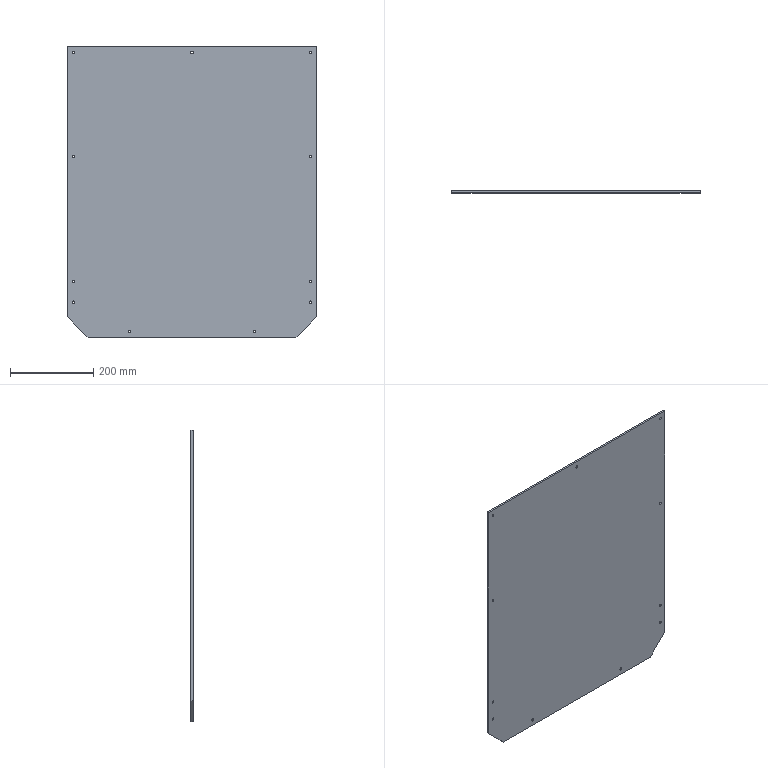Part | SolidWorks | features Extrusion 1, ICE 1 | 1 solid | 30 faces | box 600 x 5 x 700 mm | volume 2085945 mm3 | cylinder 22 | plane 8 | commonest cylinder face diameters 6 x22
STEP:
#1=CARTESIAN_POINT('',(300.,0.,-12.));
#2=VERTEX_POINT('',#1);
#3=CARTESIAN_POINT('',(300.,0.,-18.));
#4=VERTEX_POINT('',#3);
#5=CARTESIAN_POINT('',(300.,0.,-15.));
#6=DIRECTION('',(0.,-1.,0.));
#7=DIRECTION('',(0.,0.,-1.));
#8=AXIS2_PLACEMENT_3D('',#5,#6,#7);
#9=CIRCLE('',#8,3.);
#10=EDGE_CURVE('',#2,#4,#9,.T.);
#11=ORIENTED_EDGE('',*,*,#10,.T.);
#12=CARTESIAN_POINT('',(300.,5.,-18.));
#13=VERTEX_POINT('',#12);
#14=CARTESIAN_POINT('',(300.,-5.,-18.));
#15=DIRECTION('',(0.,1.,0.));
#16=VECTOR('',#15,1000.);
#17=LINE('',#14,#16);
#18=EDGE_CURVE('',#4,#13,#17,.T.);
#19=ORIENTED_EDGE('',*,*,#18,.T.);
#20=CARTESIAN_POINT('',(300.,5.,-12.));
#21=VERTEX_POINT('',#20);
#22=CARTESIAN_POINT('',(300.,5.,-15.));
#23=DIRECTION('',(0.,1.,0.));
#24=DIRECTION('',(0.,0.,1.));
#25=AXIS2_PLACEMENT_3D('',#22,#23,#24);
#26=CIRCLE('',#25,3.);
#27=EDGE_CURVE('',#13,#21,#26,.T.);
#28=ORIENTED_EDGE('',*,*,#27,.T.);
#29=CARTESIAN_POINT('',(300.,-5.,-12.));
#30=DIRECTION('',(0.,1.,0.));
#31=VECTOR('',#30,1000.);
#32=LINE('',#29,#31);
#33=EDGE_CURVE('',#2,#21,#32,.T.);
#34=ORIENTED_EDGE('',*,*,#33,.F.);
#35=EDGE_LOOP('',(#11,#19,#28,#34));
#36=FACE_OUTER_BOUND('',#35,.T.);
#37=CARTESIAN_POINT('',(300.,-5.,-15.));
#38=DIRECTION('',(0.,1.,0.));
#39=DIRECTION('',(0.,0.,1.));
#40=AXIS2_PLACEMENT_3D('',#37,#38,#39);
#41=CYLINDRICAL_SURFACE('',#40,3.);
#42=ADVANCED_FACE('',(#36),#41,.F.);
#43=CARTESIAN_POINT('',(450.,0.,-682.));
#44=VERTEX_POINT('',#43);
#45=CARTESIAN_POINT('',(450.,0.,-688.));
#46=VERTEX_POINT('',#45);
#47=CARTESIAN_POINT('',(450.,0.,-685.));
#48=DIRECTION('',(0.,-1.,0.));
#49=DIRECTION('',(0.,0.,-1.));
#50=AXIS2_PLACEMENT_3D('',#47,#48,#49);
#51=CIRCLE('',#50,3.);
#52=EDGE_CURVE('',#44,#46,#51,.T.);
#53=ORIENTED_EDGE('',*,*,#52,.T.);
#54=CARTESIAN_POINT('',(450.,5.,-688.));
#55=VERTEX_POINT('',#54);
#56=CARTESIAN_POINT('',(450.,-5.,-688.));
#57=DIRECTION('',(0.,1.,0.));
#58=VECTOR('',#57,1000.);
#59=LINE('',#56,#58);
#60=EDGE_CURVE('',#46,#55,#59,.T.);
#61=ORIENTED_EDGE('',*,*,#60,.T.);
#62=CARTESIAN_POINT('',(450.,5.,-682.));
#63=VERTEX_POINT('',#62);
#64=CARTESIAN_POINT('',(450.,5.,-685.));
#65=DIRECTION('',(0.,1.,0.));
#66=DIRECTION('',(0.,0.,-1.));
#67=AXIS2_PLACEMENT_3D('',#64,#65,#66);
#68=CIRCLE('',#67,3.);
#69=EDGE_CURVE('',#55,#63,#68,.T.);
#70=ORIENTED_EDGE('',*,*,#69,.T.);
#71=CARTESIAN_POINT('',(450.,-5.,-682.));
#72=DIRECTION('',(0.,1.,0.));
#73=VECTOR('',#72,1000.);
#74=LINE('',#71,#73);
#75=EDGE_CURVE('',#44,#63,#74,.T.);
#76=ORIENTED_EDGE('',*,*,#75,.F.);
#77=EDGE_LOOP('',(#53,#61,#70,#76));
#78=FACE_OUTER_BOUND('',#77,.T.);
#79=CARTESIAN_POINT('',(450.,-5.,-685.));
#80=DIRECTION('',(0.,1.,0.));
#81=DIRECTION('',(0.,0.,1.));
#82=AXIS2_PLACEMENT_3D('',#79,#80,#81);
#83=CYLINDRICAL_SURFACE('',#82,3.);
#84=ADVANCED_FACE('',(#78),#83,.F.);
#85=CARTESIAN_POINT('',(585.,0.,-612.));
#86=VERTEX_POINT('',#85);
#87=CARTESIAN_POINT('',(585.,0.,-618.));
#88=VERTEX_POINT('',#87);
#89=CARTESIAN_POINT('',(585.,0.,-615.));
#90=DIRECTION('',(0.,-1.,0.));
#91=DIRECTION('',(0.,0.,-1.));
#92=AXIS2_PLACEMENT_3D('',#89,#90,#91);
#93=CIRCLE('',#92,3.);
#94=EDGE_CURVE('',#86,#88,#93,.T.);
#95=ORIENTED_EDGE('',*,*,#94,.T.);
#96=CARTESIAN_POINT('',(585.,5.,-618.));
#97=VERTEX_POINT('',#96);
#98=CARTESIAN_POINT('',(585.,-5.,-618.));
#99=DIRECTION('',(0.,1.,0.));
#100=VECTOR('',#99,1000.);
#101=LINE('',#98,#100);
#102=EDGE_CURVE('',#88,#97,#101,.T.);
#103=ORIENTED_EDGE('',*,*,#102,.T.);
#104=CARTESIAN_POINT('',(585.,5.,-612.));
#105=VERTEX_POINT('',#104);
#106=CARTESIAN_POINT('',(585.,5.,-615.));
#107=DIRECTION('',(0.,1.,0.));
#108=DIRECTION('',(0.,0.,-1.));
#109=AXIS2_PLACEMENT_3D('',#106,#107,#108);
#110=CIRCLE('',#109,3.);
#111=EDGE_CURVE('',#97,#105,#110,.T.);
#112=ORIENTED_EDGE('',*,*,#111,.T.);
#113=CARTESIAN_POINT('',(585.,-5.,-612.));
#114=DIRECTION('',(0.,1.,0.));
#115=VECTOR('',#114,1000.);
#116=LINE('',#113,#115);
#117=EDGE_CURVE('',#86,#105,#116,.T.);
#118=ORIENTED_EDGE('',*,*,#117,.F.);
#119=EDGE_LOOP('',(#95,#103,#112,#118));
#120=FACE_OUTER_BOUND('',#119,.T.);
#121=CARTESIAN_POINT('',(585.,-5.,-615.));
#122=DIRECTION('',(0.,1.,0.));
#123=DIRECTION('',(0.,0.,1.));
#124=AXIS2_PLACEMENT_3D('',#121,#122,#123);
#125=CYLINDRICAL_SURFACE('',#124,3.);
#126=ADVANCED_FACE('',(#120),#125,.F.);
#127=CARTESIAN_POINT('',(585.,0.,-562.));
#128=VERTEX_POINT('',#127);
#129=CARTESIAN_POINT('',(585.,0.,-568.));
#130=VERTEX_POINT('',#129);
#131=CARTESIAN_POINT('',(585.,0.,-565.));
#132=DIRECTION('',(0.,-1.,0.));
#133=DIRECTION('',(0.,0.,-1.));
#134=AXIS2_PLACEMENT_3D('',#131,#132,#133);
#135=CIRCLE('',#134,3.);
#136=EDGE_CURVE('',#128,#130,#135,.T.);
#137=ORIENTED_EDGE('',*,*,#136,.T.);
#138=CARTESIAN_POINT('',(585.,5.,-568.));
#139=VERTEX_POINT('',#138);
#140=CARTESIAN_POINT('',(585.,-5.,-568.));
#141=DIRECTION('',(0.,1.,0.));
#142=VECTOR('',#141,1000.);
#143=LINE('',#140,#142);
#144=EDGE_CURVE('',#130,#139,#143,.T.);
#145=ORIENTED_EDGE('',*,*,#144,.T.);
#146=CARTESIAN_POINT('',(585.,5.,-562.));
#147=VERTEX_POINT('',#146);
#148=CARTESIAN_POINT('',(585.,5.,-565.));
#149=DIRECTION('',(0.,1.,0.));
#150=DIRECTION('',(0.,0.,-1.));
#151=AXIS2_PLACEMENT_3D('',#148,#149,#150);
#152=CIRCLE('',#151,3.);
#153=EDGE_CURVE('',#139,#147,#152,.T.);
#154=ORIENTED_EDGE('',*,*,#153,.T.);
#155=CARTESIAN_POINT('',(585.,-5.,-562.));
#156=DIRECTION('',(0.,1.,0.));
#157=VECTOR('',#156,1000.);
#158=LINE('',#155,#157);
#159=EDGE_CURVE('',#128,#147,#158,.T.);
#160=ORIENTED_EDGE('',*,*,#159,.F.);
#161=EDGE_LOOP('',(#137,#145,#154,#160));
#162=FACE_OUTER_BOUND('',#161,.T.);
#163=CARTESIAN_POINT('',(585.,-5.,-565.));
#164=DIRECTION('',(0.,1.,0.));
#165=DIRECTION('',(0.,0.,1.));
#166=AXIS2_PLACEMENT_3D('',#163,#164,#165);
#167=CYLINDRICAL_SURFACE('',#166,3.);
#168=ADVANCED_FACE('',(#162),#167,.F.);
#169=CARTESIAN_POINT('',(585.,0.,-262.));
#170=VERTEX_POINT('',#169);
#171=CARTESIAN_POINT('',(585.,0.,-268.));
#172=VERTEX_POINT('',#171);
#173=CARTESIAN_POINT('',(585.,0.,-265.));
#174=DIRECTION('',(0.,-1.,0.));
#175=DIRECTION('',(0.,0.,-1.));
#176=AXIS2_PLACEMENT_3D('',#173,#174,#175);
#177=CIRCLE('',#176,3.);
#178=EDGE_CURVE('',#170,#172,#177,.T.);
#179=ORIENTED_EDGE('',*,*,#178,.T.);
#180=CARTESIAN_POINT('',(585.,5.,-268.));
#181=VERTEX_POINT('',#180);
#182=CARTESIAN_POINT('',(585.,-5.,-268.));
#183=DIRECTION('',(0.,1.,0.));
#184=VECTOR('',#183,1000.);
#185=LINE('',#182,#184);
#186=EDGE_CURVE('',#172,#181,#185,.T.);
#187=ORIENTED_EDGE('',*,*,#186,.T.);
#188=CARTESIAN_POINT('',(585.,5.,-262.));
#189=VERTEX_POINT('',#188);
#190=CARTESIAN_POINT('',(585.,5.,-265.));
#191=DIRECTION('',(0.,1.,0.));
#192=DIRECTION('',(0.,0.,-1.));
#193=AXIS2_PLACEMENT_3D('',#190,#191,#192);
#194=CIRCLE('',#193,3.);
#195=EDGE_CURVE('',#181,#189,#194,.T.);
#196=ORIENTED_EDGE('',*,*,#195,.T.);
#197=CARTESIAN_POINT('',(585.,-5.,-262.));
#198=DIRECTION('',(0.,1.,0.));
#199=VECTOR('',#198,1000.);
#200=LINE('',#197,#199);
#201=EDGE_CURVE('',#170,#189,#200,.T.);
#202=ORIENTED_EDGE('',*,*,#201,.F.);
#203=EDGE_LOOP('',(#179,#187,#196,#202));
#204=FACE_OUTER_BOUND('',#203,.T.);
#205=CARTESIAN_POINT('',(585.,-5.,-265.));
#206=DIRECTION('',(0.,1.,0.));
#207=DIRECTION('',(0.,0.,1.));
#208=AXIS2_PLACEMENT_3D('',#205,#206,#207);
#209=CYLINDRICAL_SURFACE('',#208,3.);
#210=ADVANCED_FACE('',(#204),#209,.F.);
#211=CARTESIAN_POINT('',(585.,0.,-12.));
#212=VERTEX_POINT('',#211);
#213=CARTESIAN_POINT('',(585.,0.,-18.));
#214=VERTEX_POINT('',#213);
#215=CARTESIAN_POINT('',(585.,0.,-15.));
#216=DIRECTION('',(0.,-1.,0.));
#217=DIRECTION('',(0.,0.,-1.));
#218=AXIS2_PLACEMENT_3D('',#215,#216,#217);
#219=CIRCLE('',#218,3.);
#220=EDGE_CURVE('',#212,#214,#219,.T.);
#221=ORIENTED_EDGE('',*,*,#220,.T.);
#222=CARTESIAN_POINT('',(585.,5.,-18.));
#223=VERTEX_POINT('',#222);
#224=CARTESIAN_POINT('',(585.,-5.,-18.));
#225=DIRECTION('',(0.,1.,0.));
#226=VECTOR('',#225,1000.);
#227=LINE('',#224,#226);
#228=EDGE_CURVE('',#214,#223,#227,.T.);
#229=ORIENTED_EDGE('',*,*,#228,.T.);
#230=CARTESIAN_POINT('',(585.,5.,-12.));
#231=VERTEX_POINT('',#230);
#232=CARTESIAN_POINT('',(585.,5.,-15.));
#233=DIRECTION('',(0.,1.,0.));
#234=DIRECTION('',(0.,0.,-1.));
#235=AXIS2_PLACEMENT_3D('',#232,#233,#234);
#236=CIRCLE('',#235,3.);
#237=EDGE_CURVE('',#223,#231,#236,.T.);
#238=ORIENTED_EDGE('',*,*,#237,.T.);
#239=CARTESIAN_POINT('',(585.,-5.,-12.));
#240=DIRECTION('',(0.,1.,0.));
#241=VECTOR('',#240,1000.);
#242=LINE('',#239,#241);
#243=EDGE_CURVE('',#212,#231,#242,.T.);
#244=ORIENTED_EDGE('',*,*,#243,.F.);
#245=EDGE_LOOP('',(#221,#229,#238,#244));
#246=FACE_OUTER_BOUND('',#245,.T.);
#247=CARTESIAN_POINT('',(585.,-5.,-15.));
#248=DIRECTION('',(0.,1.,0.));
#249=DIRECTION('',(0.,0.,1.));
#250=AXIS2_PLACEMENT_3D('',#247,#248,#249);
#251=CYLINDRICAL_SURFACE('',#250,3.);
#252=ADVANCED_FACE('',(#246),#251,.F.);
#253=CARTESIAN_POINT('',(150.,0.,-682.));
#254=VERTEX_POINT('',#253);
#255=CARTESIAN_POINT('',(150.,0.,-688.));
#256=VERTEX_POINT('',#255);
#257=CARTESIAN_POINT('',(150.,0.,-685.));
#258=DIRECTION('',(0.,-1.,0.));
#259=DIRECTION('',(0.,0.,-1.));
#260=AXIS2_PLACEMENT_3D('',#257,#258,#259);
#261=CIRCLE('',#260,3.);
#262=EDGE_CURVE('',#254,#256,#261,.T.);
#263=ORIENTED_EDGE('',*,*,#262,.T.);
#264=CARTESIAN_POINT('',(150.,5.,-688.));
#265=VERTEX_POINT('',#264);
#266=CARTESIAN_POINT('',(150.,-5.,-688.));
#267=DIRECTION('',(0.,1.,0.));
#268=VECTOR('',#267,1000.);
#269=LINE('',#266,#268);
#270=EDGE_CURVE('',#256,#265,#269,.T.);
#271=ORIENTED_EDGE('',*,*,#270,.T.);
#272=CARTESIAN_POINT('',(150.,5.,-682.));
#273=VERTEX_POINT('',#272);
#274=CARTESIAN_POINT('',(150.,5.,-685.));
#275=DIRECTION('',(0.,1.,0.));
#276=DIRECTION('',(0.,0.,1.));
#277=AXIS2_PLACEMENT_3D('',#274,#275,#276);
#278=CIRCLE('',#277,3.);
#279=EDGE_CURVE('',#265,#273,#278,.T.);
#280=ORIENTED_EDGE('',*,*,#279,.T.);
#281=CARTESIAN_POINT('',(150.,-5.,-682.));
#282=DIRECTION('',(0.,1.,0.));
#283=VECTOR('',#282,1000.);
#284=LINE('',#281,#283);
#285=EDGE_CURVE('',#254,#273,#284,.T.);
#286=ORIENTED_EDGE('',*,*,#285,.F.);
#287=EDGE_LOOP('',(#263,#271,#280,#286));
#288=FACE_OUTER_BOUND('',#287,.T.);
#289=CARTESIAN_POINT('',(150.,-5.,-685.));
#290=DIRECTION('',(0.,1.,0.));
#291=DIRECTION('',(0.,0.,1.));
#292=AXIS2_PLACEMENT_3D('',#289,#290,#291);
#293=CYLINDRICAL_SURFACE('',#292,3.);
#294=ADVANCED_FACE('',(#288),#293,.F.);
#295=CARTESIAN_POINT('',(15.,0.,-612.));
#296=VERTEX_POINT('',#295);
#297=CARTESIAN_POINT('',(15.,0.,-618.));
#298=VERTEX_POINT('',#297);
#299=CARTESIAN_POINT('',(15.,0.,-615.));
#300=DIRECTION('',(0.,-1.,0.));
#301=DIRECTION('',(0.,0.,-1.));
#302=AXIS2_PLACEMENT_3D('',#299,#300,#301);
#303=CIRCLE('',#302,3.);
#304=EDGE_CURVE('',#296,#298,#303,.T.);
#305=ORIENTED_EDGE('',*,*,#304,.T.);
#306=CARTESIAN_POINT('',(15.,5.,-618.));
#307=VERTEX_POINT('',#306);
#308=CARTESIAN_POINT('',(15.,-5.,-618.));
#309=DIRECTION('',(0.,1.,0.));
#310=VECTOR('',#309,1000.);
#311=LINE('',#308,#310);
#312=EDGE_CURVE('',#298,#307,#311,.T.);
#313=ORIENTED_EDGE('',*,*,#312,.T.);
#314=CARTESIAN_POINT('',(15.,5.,-612.));
#315=VERTEX_POINT('',#314);
#316=CARTESIAN_POINT('',(15.,5.,-615.));
#317=DIRECTION('',(0.,1.,0.));
#318=DIRECTION('',(0.,0.,1.));
#319=AXIS2_PLACEMENT_3D('',#316,#317,#318);
#320=CIRCLE('',#319,3.);
#321=EDGE_CURVE('',#307,#315,#320,.T.);
#322=ORIENTED_EDGE('',*,*,#321,.T.);
#323=CARTESIAN_POINT('',(15.,-5.,-612.));
#324=DIRECTION('',(0.,1.,0.));
#325=VECTOR('',#324,1000.);
#326=LINE('',#323,#325);
#327=EDGE_CURVE('',#296,#315,#326,.T.);
#328=ORIENTED_EDGE('',*,*,#327,.F.);
#329=EDGE_LOOP('',(#305,#313,#322,#328));
#330=FACE_OUTER_BOUND('',#329,.T.);
#331=CARTESIAN_POINT('',(15.,-5.,-615.));
#332=DIRECTION('',(0.,1.,0.));
#333=DIRECTION('',(0.,0.,1.));
#334=AXIS2_PLACEMENT_3D('',#331,#332,#333);
#335=CYLINDRICAL_SURFACE('',#334,3.);
#336=ADVANCED_FACE('',(#330),#335,.F.);
#337=CARTESIAN_POINT('',(15.,0.,-562.));
#338=VERTEX_POINT('',#337);
#339=CARTESIAN_POINT('',(15.,0.,-568.));
#340=VERTEX_POINT('',#339);
#341=CARTESIAN_POINT('',(15.,0.,-565.));
#342=DIRECTION('',(0.,-1.,0.));
#343=DIRECTION('',(0.,0.,-1.));
#344=AXIS2_PLACEMENT_3D('',#341,#342,#343);
#345=CIRCLE('',#344,3.);
#346=EDGE_CURVE('',#338,#340,#345,.T.);
#347=ORIENTED_EDGE('',*,*,#346,.T.);
#348=CARTESIAN_POINT('',(15.,5.,-568.));
#349=VERTEX_POINT('',#348);
#350=CARTESIAN_POINT('',(15.,-5.,-568.));
#351=DIRECTION('',(0.,1.,0.));
#352=VECTOR('',#351,1000.);
#353=LINE('',#350,#352);
#354=EDGE_CURVE('',#340,#349,#353,.T.);
#355=ORIENTED_EDGE('',*,*,#354,.T.);
#356=CARTESIAN_POINT('',(15.,5.,-562.));
#357=VERTEX_POINT('',#356);
#358=CARTESIAN_POINT('',(15.,5.,-565.));
#359=DIRECTION('',(0.,1.,0.));
#360=DIRECTION('',(0.,0.,1.));
#361=AXIS2_PLACEMENT_3D('',#358,#359,#360);
#362=CIRCLE('',#361,3.);
#363=EDGE_CURVE('',#349,#357,#362,.T.);
#364=ORIENTED_EDGE('',*,*,#363,.T.);
#365=CARTESIAN_POINT('',(15.,-5.,-562.));
#366=DIRECTION('',(0.,1.,0.));
#367=VECTOR('',#366,1000.);
#368=LINE('',#365,#367);
#369=EDGE_CURVE('',#338,#357,#368,.T.);
#370=ORIENTED_EDGE('',*,*,#369,.F.);
#371=EDGE_LOOP('',(#347,#355,#364,#370));
#372=FACE_OUTER_BOUND('',#371,.T.);
#373=CARTESIAN_POINT('',(15.,-5.,-565.));
#374=DIRECTION('',(0.,1.,0.));
#375=DIRECTION('',(0.,0.,1.));
#376=AXIS2_PLACEMENT_3D('',#373,#374,#375);
#377=CYLINDRICAL_SURFACE('',#376,3.);
#378=ADVANCED_FACE('',(#372),#377,.F.);
#379=CARTESIAN_POINT('',(15.,0.,-262.));
#380=VERTEX_POINT('',#379);
#381=CARTESIAN_POINT('',(15.,0.,-268.));
#382=VERTEX_POINT('',#381);
#383=CARTESIAN_POINT('',(15.,0.,-265.));
#384=DIRECTION('',(0.,-1.,0.));
#385=DIRECTION('',(0.,0.,-1.));
#386=AXIS2_PLACEMENT_3D('',#383,#384,#385);
#387=CIRCLE('',#386,3.);
#388=EDGE_CURVE('',#380,#382,#387,.T.);
#389=ORIENTED_EDGE('',*,*,#388,.T.);
#390=CARTESIAN_POINT('',(15.,5.,-268.));
#391=VERTEX_POINT('',#390);
#392=CARTESIAN_POINT('',(15.,-5.,-268.));
#393=DIRECTION('',(0.,1.,0.));
#394=VECTOR('',#393,1000.);
#395=LINE('',#392,#394);
#396=EDGE_CURVE('',#382,#391,#395,.T.);
#397=ORIENTED_EDGE('',*,*,#396,.T.);
#398=CARTESIAN_POINT('',(15.,5.,-262.));
#399=VERTEX_POINT('',#398);
#400=CARTESIAN_POINT('',(15.,5.,-265.));
#401=DIRECTION('',(0.,1.,0.));
#402=DIRECTION('',(0.,0.,1.));
#403=AXIS2_PLACEMENT_3D('',#400,#401,#402);
#404=CIRCLE('',#403,3.);
#405=EDGE_CURVE('',#391,#399,#404,.T.);
#406=ORIENTED_EDGE('',*,*,#405,.T.);
#407=CARTESIAN_POINT('',(15.,-5.,-262.));
#408=DIRECTION('',(0.,1.,0.));
#409=VECTOR('',#408,1000.);
#410=LINE('',#407,#409);
#411=EDGE_CURVE('',#380,#399,#410,.T.);
#412=ORIENTED_EDGE('',*,*,#411,.F.);
#413=EDGE_LOOP('',(#389,#397,#406,#412));
#414=FACE_OUTER_BOUND('',#413,.T.);
#415=CARTESIAN_POINT('',(15.,-5.,-265.));
#416=DIRECTION('',(0.,1.,0.));
#417=DIRECTION('',(0.,0.,1.));
#418=AXIS2_PLACEMENT_3D('',#415,#416,#417);
#419=CYLINDRICAL_SURFACE('',#418,3.);
#420=ADVANCED_FACE('',(#414),#419,.F.);
#421=CARTESIAN_POINT('',(15.,0.,-12.));
#422=VERTEX_POINT('',#421);
#423=CARTESIAN_POINT('',(15.,0.,-18.));
#424=VERTEX_POINT('',#423);
#425=CARTESIAN_POINT('',(15.,0.,-15.));
#426=DIRECTION('',(0.,-1.,0.));
#427=DIRECTION('',(0.,0.,-1.));
#428=AXIS2_PLACEMENT_3D('',#425,#426,#427);
#429=CIRCLE('',#428,3.);
#430=EDGE_CURVE('',#422,#424,#429,.T.);
#431=ORIENTED_EDGE('',*,*,#430,.T.);
#432=CARTESIAN_POINT('',(15.,5.,-18.));
#433=VERTEX_POINT('',#432);
#434=CARTESIAN_POINT('',(15.,-5.,-18.));
#435=DIRECTION('',(0.,1.,0.));
#436=VECTOR('',#435,1000.);
#437=LINE('',#434,#436);
#438=EDGE_CURVE('',#424,#433,#437,.T.);
#439=ORIENTED_EDGE('',*,*,#438,.T.);
#440=CARTESIAN_POINT('',(15.,5.,-12.));
#441=VERTEX_POINT('',#440);
#442=CARTESIAN_POINT('',(15.,5.,-15.));
#443=DIRECTION('',(0.,1.,0.));
#444=DIRECTION('',(0.,0.,1.));
#445=AXIS2_PLACEMENT_3D('',#442,#443,#444);
#446=CIRCLE('',#445,3.);
#447=EDGE_CURVE('',#433,#441,#446,.T.);
#448=ORIENTED_EDGE('',*,*,#447,.T.);
#449=CARTESIAN_POINT('',(15.,-5.,-12.));
#450=DIRECTION('',(0.,1.,0.));
#451=VECTOR('',#450,1000.);
#452=LINE('',#449,#451);
#453=EDGE_CURVE('',#422,#441,#452,.T.);
#454=ORIENTED_EDGE('',*,*,#453,.F.);
#455=EDGE_LOOP('',(#431,#439,#448,#454));
#456=FACE_OUTER_BOUND('',#455,.T.);
#457=CARTESIAN_POINT('',(15.,-5.,-15.));
#458=DIRECTION('',(0.,1.,0.));
#459=DIRECTION('',(0.,0.,1.));
#460=AXIS2_PLACEMENT_3D('',#457,#458,#459);
#461=CYLINDRICAL_SURFACE('',#460,3.);
#462=ADVANCED_FACE('',(#456),#461,.F.);
#463=CARTESIAN_POINT('',(0.,0.,-650.));
#464=VERTEX_POINT('',#463);
#465=CARTESIAN_POINT('',(0.,0.,0.));
#466=VERTEX_POINT('',#465);
#467=CARTESIAN_POINT('',(0.,0.,0.));
#468=DIRECTION('',(0.,0.,1.));
#469=VECTOR('',#468,1000.);
#470=LINE('',#467,#469);
#471=EDGE_CURVE('',#464,#466,#470,.T.);
#472=ORIENTED_EDGE('',*,*,#471,.T.);
#473=CARTESIAN_POINT('',(0.,5.,0.));
#474=VERTEX_POINT('',#473);
#475=CARTESIAN_POINT('',(0.,5.,0.));
#476=DIRECTION('',(0.,-1.,0.));
#477=VECTOR('',#476,1000.);
#478=LINE('',#475,#477);
#479=EDGE_CURVE('',#474,#466,#478,.T.);
#480=ORIENTED_EDGE('',*,*,#479,.F.);
#481=CARTESIAN_POINT('',(0.,5.,-650.));
#482=VERTEX_POINT('',#481);
#483=CARTESIAN_POINT('',(0.,5.,0.));
#484=DIRECTION('',(0.,0.,1.));
#485=VECTOR('',#484,1000.);
#486=LINE('',#483,#485);
#487=EDGE_CURVE('',#482,#474,#486,.T.);
#488=ORIENTED_EDGE('',*,*,#487,.F.);
#489=CARTESIAN_POINT('',(0.,5.,-650.));
#490=DIRECTION('',(0.,-1.,0.));
#491=VECTOR('',#490,1000.);
#492=LINE('',#489,#491);
#493=EDGE_CURVE('',#482,#464,#492,.T.);
#494=ORIENTED_EDGE('',*,*,#493,.T.);
#495=EDGE_LOOP('',(#472,#480,#488,#494));
#496=FACE_OUTER_BOUND('',#495,.T.);
#497=CARTESIAN_POINT('',(0.,5.,0.));
#498=DIRECTION('',(1.,0.,0.));
#499=DIRECTION('',(0.,0.,-1.));
#500=AXIS2_PLACEMENT_3D('',#497,#498,#499);
#501=PLANE('',#500);
#502=ADVANCED_FACE('',(#496),#501,.F.);
#503=CARTESIAN_POINT('',(600.,0.,0.));
#504=VERTEX_POINT('',#503);
#505=CARTESIAN_POINT('',(0.,0.,0.));
#506=DIRECTION('',(1.,0.,0.));
#507=VECTOR('',#506,1000.);
#508=LINE('',#505,#507);
#509=EDGE_CURVE('',#466,#504,#508,.T.);
#510=ORIENTED_EDGE('',*,*,#509,.T.);
#511=CARTESIAN_POINT('',(600.,5.,0.));
#512=VERTEX_POINT('',#511);
#513=CARTESIAN_POINT('',(600.,5.,0.));
#514=DIRECTION('',(0.,-1.,0.));
#515=VECTOR('',#514,1000.);
#516=LINE('',#513,#515);
#517=EDGE_CURVE('',#512,#504,#516,.T.);
#518=ORIENTED_EDGE('',*,*,#517,.F.);
#519=CARTESIAN_POINT('',(0.,5.,0.));
#520=DIRECTION('',(1.,0.,0.));
#521=VECTOR('',#520,1000.);
#522=LINE('',#519,#521);
#523=EDGE_CURVE('',#474,#512,#522,.T.);
#524=ORIENTED_EDGE('',*,*,#523,.F.);
#525=ORIENTED_EDGE('',*,*,#479,.T.);
#526=EDGE_LOOP('',(#510,#518,#524,#525));
#527=FACE_OUTER_BOUND('',#526,.T.);
#528=CARTESIAN_POINT('',(0.,5.,0.));
#529=DIRECTION('',(0.,0.,-1.));
#530=DIRECTION('',(-1.,0.,0.));
#531=AXIS2_PLACEMENT_3D('',#528,#529,#530);
#532=PLANE('',#531);
#533=ADVANCED_FACE('',(#527),#532,.F.);
#534=CARTESIAN_POINT('',(600.,0.,-650.));
#535=VERTEX_POINT('',#534);
#536=CARTESIAN_POINT('',(600.,0.,0.));
#537=DIRECTION('',(0.,0.,-1.));
#538=VECTOR('',#537,1000.);
#539=LINE('',#536,#538);
#540=EDGE_CURVE('',#504,#535,#539,.T.);
#541=ORIENTED_EDGE('',*,*,#540,.T.);
#542=CARTESIAN_POINT('',(600.,5.,-650.));
#543=VERTEX_POINT('',#542);
#544=CARTESIAN_POINT('',(600.,5.,-650.));
#545=DIRECTION('',(0.,-1.,0.));
#546=VECTOR('',#545,1000.);
#547=LINE('',#544,#546);
#548=EDGE_CURVE('',#543,#535,#547,.T.);
#549=ORIENTED_EDGE('',*,*,#548,.F.);
#550=CARTESIAN_POINT('',(600.,5.,0.));
#551=DIRECTION('',(0.,0.,-1.));
#552=VECTOR('',#551,1000.);
#553=LINE('',#550,#552);
#554=EDGE_CURVE('',#512,#543,#553,.T.);
#555=ORIENTED_EDGE('',*,*,#554,.F.);
#556=ORIENTED_EDGE('',*,*,#517,.T.);
#557=EDGE_LOOP('',(#541,#549,#555,#556));
#558=FACE_OUTER_BOUND('',#557,.T.);
#559=CARTESIAN_POINT('',(600.,5.,0.));
#560=DIRECTION('',(-1.,0.,0.));
#561=DIRECTION('',(0.,0.,1.));
#562=AXIS2_PLACEMENT_3D('',#559,#560,#561);
#563=PLANE('',#562);
#564=ADVANCED_FACE('',(#558),#563,.F.);
#565=CARTESIAN_POINT('',(550.,0.,-700.));
#566=VERTEX_POINT('',#565);
#567=CARTESIAN_POINT('',(550.,0.,-700.));
#568=DIRECTION('',(-0.7071,0.,-0.7071));
#569=VECTOR('',#568,1000.);
#570=LINE('',#567,#569);
#571=EDGE_CURVE('',#535,#566,#570,.T.);
#572=ORIENTED_EDGE('',*,*,#571,.T.);
#573=CARTESIAN_POINT('',(550.,5.,-700.));
#574=VERTEX_POINT('',#573);
#575=CARTESIAN_POINT('',(550.,5.,-700.));
#576=DIRECTION('',(0.,-1.,0.));
#577=VECTOR('',#576,1000.);
#578=LINE('',#575,#577);
#579=EDGE_CURVE('',#574,#566,#578,.T.);
#580=ORIENTED_EDGE('',*,*,#579,.F.);
#581=CARTESIAN_POINT('',(550.,5.,-700.));
#582=DIRECTION('',(-0.7071,0.,-0.7071));
#583=VECTOR('',#582,1000.);
#584=LINE('',#581,#583);
#585=EDGE_CURVE('',#543,#574,#584,.T.);
#586=ORIENTED_EDGE('',*,*,#585,.F.);
#587=ORIENTED_EDGE('',*,*,#548,.T.);
#588=EDGE_LOOP('',(#572,#580,#586,#587));
#589=FACE_OUTER_BOUND('',#588,.T.);
#590=CARTESIAN_POINT('',(550.,5.,-700.));
#591=DIRECTION('',(-0.7071,0.,0.7071));
#592=DIRECTION('',(0.7071,0.,0.7071));
#593=AXIS2_PLACEMENT_3D('',#590,#591,#592);
#594=PLANE('',#593);
#595=ADVANCED_FACE('',(#589),#594,.F.);
#596=CARTESIAN_POINT('',(50.,0.,-700.));
#597=VERTEX_POINT('',#596);
#598=CARTESIAN_POINT('',(50.,0.,-700.));
#599=DIRECTION('',(-1.,0.,0.));
#600=VECTOR('',#599,1000.);
#601=LINE('',#598,#600);
#602=EDGE_CURVE('',#566,#597,#601,.T.);
#603=ORIENTED_EDGE('',*,*,#602,.T.);
#604=CARTESIAN_POINT('',(50.,5.,-700.));
#605=VERTEX_POINT('',#604);
#606=CARTESIAN_POINT('',(50.,5.,-700.));
#607=DIRECTION('',(0.,-1.,0.));
#608=VECTOR('',#607,1000.);
#609=LINE('',#606,#608);
#610=EDGE_CURVE('',#605,#597,#609,.T.);
#611=ORIENTED_EDGE('',*,*,#610,.F.);
#612=CARTESIAN_POINT('',(50.,5.,-700.));
#613=DIRECTION('',(-1.,0.,0.));
#614=VECTOR('',#613,1000.);
#615=LINE('',#612,#614);
#616=EDGE_CURVE('',#574,#605,#615,.T.);
#617=ORIENTED_EDGE('',*,*,#616,.F.);
#618=ORIENTED_EDGE('',*,*,#579,.T.);
#619=EDGE_LOOP('',(#603,#611,#617,#618));
#620=FACE_OUTER_BOUND('',#619,.T.);
#621=CARTESIAN_POINT('',(50.,5.,-700.));
#622=DIRECTION('',(0.,0.,1.));
#623=DIRECTION('',(1.,0.,0.));
#624=AXIS2_PLACEMENT_3D('',#621,#622,#623);
#625=PLANE('',#624);
#626=ADVANCED_FACE('',(#620),#625,.F.);
#627=CARTESIAN_POINT('',(0.,0.,-650.));
#628=DIRECTION('',(-0.7071,0.,0.7071));
#629=VECTOR('',#628,1000.);
#630=LINE('',#627,#629);
#631=EDGE_CURVE('',#597,#464,#630,.T.);
#632=ORIENTED_EDGE('',*,*,#631,.T.);
#633=ORIENTED_EDGE('',*,*,#493,.F.);
#634=CARTESIAN_POINT('',(0.,5.,-650.));
#635=DIRECTION('',(-0.7071,0.,0.7071));
#636=VECTOR('',#635,1000.);
#637=LINE('',#634,#636);
#638=EDGE_CURVE('',#605,#482,#637,.T.);
#639=ORIENTED_EDGE('',*,*,#638,.F.);
#640=ORIENTED_EDGE('',*,*,#610,.T.);
#641=EDGE_LOOP('',(#632,#633,#639,#640));
#642=FACE_OUTER_BOUND('',#641,.T.);
#643=CARTESIAN_POINT('',(0.,5.,-650.));
#644=DIRECTION('',(0.7071,0.,0.7071));
#645=DIRECTION('',(0.7071,0.,-0.7071));
#646=AXIS2_PLACEMENT_3D('',#643,#644,#645);
#647=PLANE('',#646);
#648=ADVANCED_FACE('',(#642),#647,.F.);
#649=CARTESIAN_POINT('',(300.,5.,-15.));
#650=DIRECTION('',(0.,1.,0.));
#651=DIRECTION('',(0.,0.,1.));
#652=AXIS2_PLACEMENT_3D('',#649,#650,#651);
#653=CIRCLE('',#652,3.);
#654=EDGE_CURVE('',#21,#13,#653,.T.);
#655=ORIENTED_EDGE('',*,*,#654,.F.);
#656=ORIENTED_EDGE('',*,*,#27,.F.);
#657=EDGE_LOOP('',(#655,#656));
#658=FACE_BOUND('',#657,.T.);
#659=CARTESIAN_POINT('',(450.,5.,-685.));
#660=DIRECTION('',(0.,1.,0.));
#661=DIRECTION('',(0.,0.,-1.));
#662=AXIS2_PLACEMENT_3D('',#659,#660,#661);
#663=CIRCLE('',#662,3.);
#664=EDGE_CURVE('',#63,#55,#663,.T.);
#665=ORIENTED_EDGE('',*,*,#664,.F.);
#666=ORIENTED_EDGE('',*,*,#69,.F.);
#667=EDGE_LOOP('',(#665,#666));
#668=FACE_BOUND('',#667,.T.);
#669=CARTESIAN_POINT('',(585.,5.,-615.));
#670=DIRECTION('',(0.,1.,0.));
#671=DIRECTION('',(0.,0.,-1.));
#672=AXIS2_PLACEMENT_3D('',#669,#670,#671);
#673=CIRCLE('',#672,3.);
#674=EDGE_CURVE('',#105,#97,#673,.T.);
#675=ORIENTED_EDGE('',*,*,#674,.F.);
#676=ORIENTED_EDGE('',*,*,#111,.F.);
#677=EDGE_LOOP('',(#675,#676));
#678=FACE_BOUND('',#677,.T.);
#679=CARTESIAN_POINT('',(585.,5.,-565.));
#680=DIRECTION('',(0.,1.,0.));
#681=DIRECTION('',(0.,0.,-1.));
#682=AXIS2_PLACEMENT_3D('',#679,#680,#681);
#683=CIRCLE('',#682,3.);
#684=EDGE_CURVE('',#147,#139,#683,.T.);
#685=ORIENTED_EDGE('',*,*,#684,.F.);
#686=ORIENTED_EDGE('',*,*,#153,.F.);
#687=EDGE_LOOP('',(#685,#686));
#688=FACE_BOUND('',#687,.T.);
#689=CARTESIAN_POINT('',(585.,5.,-265.));
#690=DIRECTION('',(0.,1.,0.));
#691=DIRECTION('',(0.,0.,-1.));
#692=AXIS2_PLACEMENT_3D('',#689,#690,#691);
#693=CIRCLE('',#692,3.);
#694=EDGE_CURVE('',#189,#181,#693,.T.);
#695=ORIENTED_EDGE('',*,*,#694,.F.);
#696=ORIENTED_EDGE('',*,*,#195,.F.);
#697=EDGE_LOOP('',(#695,#696));
#698=FACE_BOUND('',#697,.T.);
#699=CARTESIAN_POINT('',(585.,5.,-15.));
#700=DIRECTION('',(0.,1.,0.));
#701=DIRECTION('',(0.,0.,-1.));
#702=AXIS2_PLACEMENT_3D('',#699,#700,#701);
#703=CIRCLE('',#702,3.);
#704=EDGE_CURVE('',#231,#223,#703,.T.);
#705=ORIENTED_EDGE('',*,*,#704,.F.);
#706=ORIENTED_EDGE('',*,*,#237,.F.);
#707=EDGE_LOOP('',(#705,#706));
#708=FACE_BOUND('',#707,.T.);
#709=CARTESIAN_POINT('',(150.,5.,-685.));
#710=DIRECTION('',(0.,1.,0.));
#711=DIRECTION('',(0.,0.,1.));
#712=AXIS2_PLACEMENT_3D('',#709,#710,#711);
#713=CIRCLE('',#712,3.);
#714=EDGE_CURVE('',#273,#265,#713,.T.);
#715=ORIENTED_EDGE('',*,*,#714,.F.);
#716=ORIENTED_EDGE('',*,*,#279,.F.);
#717=EDGE_LOOP('',(#715,#716));
#718=FACE_BOUND('',#717,.T.);
#719=CARTESIAN_POINT('',(15.,5.,-615.));
#720=DIRECTION('',(0.,1.,0.));
#721=DIRECTION('',(0.,0.,1.));
#722=AXIS2_PLACEMENT_3D('',#719,#720,#721);
#723=CIRCLE('',#722,3.);
#724=EDGE_CURVE('',#315,#307,#723,.T.);
#725=ORIENTED_EDGE('',*,*,#724,.F.);
#726=ORIENTED_EDGE('',*,*,#321,.F.);
#727=EDGE_LOOP('',(#725,#726));
#728=FACE_BOUND('',#727,.T.);
#729=CARTESIAN_POINT('',(15.,5.,-565.));
#730=DIRECTION('',(0.,1.,0.));
#731=DIRECTION('',(0.,0.,1.));
#732=AXIS2_PLACEMENT_3D('',#729,#730,#731);
#733=CIRCLE('',#732,3.);
#734=EDGE_CURVE('',#357,#349,#733,.T.);
#735=ORIENTED_EDGE('',*,*,#734,.F.);
#736=ORIENTED_EDGE('',*,*,#363,.F.);
#737=EDGE_LOOP('',(#735,#736));
#738=FACE_BOUND('',#737,.T.);
#739=CARTESIAN_POINT('',(15.,5.,-265.));
#740=DIRECTION('',(0.,1.,0.));
#741=DIRECTION('',(0.,0.,1.));
#742=AXIS2_PLACEMENT_3D('',#739,#740,#741);
#743=CIRCLE('',#742,3.);
#744=EDGE_CURVE('',#399,#391,#743,.T.);
#745=ORIENTED_EDGE('',*,*,#744,.F.);
#746=ORIENTED_EDGE('',*,*,#405,.F.);
#747=EDGE_LOOP('',(#745,#746));
#748=FACE_BOUND('',#747,.T.);
#749=CARTESIAN_POINT('',(15.,5.,-15.));
#750=DIRECTION('',(0.,1.,0.));
#751=DIRECTION('',(0.,0.,1.));
#752=AXIS2_PLACEMENT_3D('',#749,#750,#751);
#753=CIRCLE('',#752,3.);
#754=EDGE_CURVE('',#441,#433,#753,.T.);
#755=ORIENTED_EDGE('',*,*,#754,.F.);
#756=ORIENTED_EDGE('',*,*,#447,.F.);
#757=EDGE_LOOP('',(#755,#756));
#758=FACE_BOUND('',#757,.T.);
#759=ORIENTED_EDGE('',*,*,#487,.T.);
#760=ORIENTED_EDGE('',*,*,#523,.T.);
#761=ORIENTED_EDGE('',*,*,#554,.T.);
#762=ORIENTED_EDGE('',*,*,#585,.T.);
#763=ORIENTED_EDGE('',*,*,#616,.T.);
#764=ORIENTED_EDGE('',*,*,#638,.T.);
#765=EDGE_LOOP('',(#759,#760,#761,#762,#763,#764));
#766=FACE_OUTER_BOUND('',#765,.T.);
#767=CARTESIAN_POINT('',(0.,5.,-700.));
#768=DIRECTION('',(0.,-1.,0.));
#769=DIRECTION('',(0.,0.,-1.));
#770=AXIS2_PLACEMENT_3D('',#767,#768,#769);
#771=PLANE('',#770);
#772=ADVANCED_FACE('',(#658,#668,#678,#688,#698,#708,#718,#728,#738,#748,#758,#766),#771,.F.);
#773=ORIENTED_EDGE('',*,*,#10,.F.);
#774=CARTESIAN_POINT('',(300.,0.,-15.));
#775=DIRECTION('',(0.,-1.,0.));
#776=DIRECTION('',(0.,0.,-1.));
#777=AXIS2_PLACEMENT_3D('',#774,#775,#776);
#778=CIRCLE('',#777,3.);
#779=EDGE_CURVE('',#4,#2,#778,.T.);
#780=ORIENTED_EDGE('',*,*,#779,.F.);
#781=EDGE_LOOP('',(#773,#780));
#782=FACE_BOUND('',#781,.T.);
#783=ORIENTED_EDGE('',*,*,#52,.F.);
#784=CARTESIAN_POINT('',(450.,0.,-685.));
#785=DIRECTION('',(0.,-1.,0.));
#786=DIRECTION('',(0.,0.,-1.));
#787=AXIS2_PLACEMENT_3D('',#784,#785,#786);
#788=CIRCLE('',#787,3.);
#789=EDGE_CURVE('',#46,#44,#788,.T.);
#790=ORIENTED_EDGE('',*,*,#789,.F.);
#791=EDGE_LOOP('',(#783,#790));
#792=FACE_BOUND('',#791,.T.);
#793=ORIENTED_EDGE('',*,*,#94,.F.);
#794=CARTESIAN_POINT('',(585.,0.,-615.));
#795=DIRECTION('',(0.,-1.,0.));
#796=DIRECTION('',(0.,0.,-1.));
#797=AXIS2_PLACEMENT_3D('',#794,#795,#796);
#798=CIRCLE('',#797,3.);
#799=EDGE_CURVE('',#88,#86,#798,.T.);
#800=ORIENTED_EDGE('',*,*,#799,.F.);
#801=EDGE_LOOP('',(#793,#800));
#802=FACE_BOUND('',#801,.T.);
#803=ORIENTED_EDGE('',*,*,#136,.F.);
#804=CARTESIAN_POINT('',(585.,0.,-565.));
#805=DIRECTION('',(0.,-1.,0.));
#806=DIRECTION('',(0.,0.,-1.));
#807=AXIS2_PLACEMENT_3D('',#804,#805,#806);
#808=CIRCLE('',#807,3.);
#809=EDGE_CURVE('',#130,#128,#808,.T.);
#810=ORIENTED_EDGE('',*,*,#809,.F.);
#811=EDGE_LOOP('',(#803,#810));
#812=FACE_BOUND('',#811,.T.);
#813=ORIENTED_EDGE('',*,*,#178,.F.);
#814=CARTESIAN_POINT('',(585.,0.,-265.));
#815=DIRECTION('',(0.,-1.,0.));
#816=DIRECTION('',(0.,0.,-1.));
#817=AXIS2_PLACEMENT_3D('',#814,#815,#816);
#818=CIRCLE('',#817,3.);
#819=EDGE_CURVE('',#172,#170,#818,.T.);
#820=ORIENTED_EDGE('',*,*,#819,.F.);
#821=EDGE_LOOP('',(#813,#820));
#822=FACE_BOUND('',#821,.T.);
#823=ORIENTED_EDGE('',*,*,#220,.F.);
#824=CARTESIAN_POINT('',(585.,0.,-15.));
#825=DIRECTION('',(0.,-1.,0.));
#826=DIRECTION('',(0.,0.,-1.));
#827=AXIS2_PLACEMENT_3D('',#824,#825,#826);
#828=CIRCLE('',#827,3.);
#829=EDGE_CURVE('',#214,#212,#828,.T.);
#830=ORIENTED_EDGE('',*,*,#829,.F.);
#831=EDGE_LOOP('',(#823,#830));
#832=FACE_BOUND('',#831,.T.);
#833=ORIENTED_EDGE('',*,*,#262,.F.);
#834=CARTESIAN_POINT('',(150.,0.,-685.));
#835=DIRECTION('',(0.,-1.,0.));
#836=DIRECTION('',(0.,0.,-1.));
#837=AXIS2_PLACEMENT_3D('',#834,#835,#836);
#838=CIRCLE('',#837,3.);
#839=EDGE_CURVE('',#256,#254,#838,.T.);
#840=ORIENTED_EDGE('',*,*,#839,.F.);
#841=EDGE_LOOP('',(#833,#840));
#842=FACE_BOUND('',#841,.T.);
#843=ORIENTED_EDGE('',*,*,#304,.F.);
#844=CARTESIAN_POINT('',(15.,0.,-615.));
#845=DIRECTION('',(0.,-1.,0.));
#846=DIRECTION('',(0.,0.,-1.));
#847=AXIS2_PLACEMENT_3D('',#844,#845,#846);
#848=CIRCLE('',#847,3.);
#849=EDGE_CURVE('',#298,#296,#848,.T.);
#850=ORIENTED_EDGE('',*,*,#849,.F.);
#851=EDGE_LOOP('',(#843,#850));
#852=FACE_BOUND('',#851,.T.);
#853=ORIENTED_EDGE('',*,*,#346,.F.);
#854=CARTESIAN_POINT('',(15.,0.,-565.));
#855=DIRECTION('',(0.,-1.,0.));
#856=DIRECTION('',(0.,0.,-1.));
#857=AXIS2_PLACEMENT_3D('',#854,#855,#856);
#858=CIRCLE('',#857,3.);
#859=EDGE_CURVE('',#340,#338,#858,.T.);
#860=ORIENTED_EDGE('',*,*,#859,.F.);
#861=EDGE_LOOP('',(#853,#860));
#862=FACE_BOUND('',#861,.T.);
#863=ORIENTED_EDGE('',*,*,#388,.F.);
#864=CARTESIAN_POINT('',(15.,0.,-265.));
#865=DIRECTION('',(0.,-1.,0.));
#866=DIRECTION('',(0.,0.,-1.));
#867=AXIS2_PLACEMENT_3D('',#864,#865,#866);
#868=CIRCLE('',#867,3.);
#869=EDGE_CURVE('',#382,#380,#868,.T.);
#870=ORIENTED_EDGE('',*,*,#869,.F.);
#871=EDGE_LOOP('',(#863,#870));
#872=FACE_BOUND('',#871,.T.);
#873=ORIENTED_EDGE('',*,*,#430,.F.);
#874=CARTESIAN_POINT('',(15.,0.,-15.));
#875=DIRECTION('',(0.,-1.,0.));
#876=DIRECTION('',(0.,0.,-1.));
#877=AXIS2_PLACEMENT_3D('',#874,#875,#876);
#878=CIRCLE('',#877,3.);
#879=EDGE_CURVE('',#424,#422,#878,.T.);
#880=ORIENTED_EDGE('',*,*,#879,.F.);
#881=EDGE_LOOP('',(#873,#880));
#882=FACE_BOUND('',#881,.T.);
#883=ORIENTED_EDGE('',*,*,#471,.F.);
#884=ORIENTED_EDGE('',*,*,#631,.F.);
#885=ORIENTED_EDGE('',*,*,#602,.F.);
#886=ORIENTED_EDGE('',*,*,#571,.F.);
#887=ORIENTED_EDGE('',*,*,#540,.F.);
#888=ORIENTED_EDGE('',*,*,#509,.F.);
#889=EDGE_LOOP('',(#883,#884,#885,#886,#887,#888));
#890=FACE_OUTER_BOUND('',#889,.T.);
#891=CARTESIAN_POINT('',(0.,0.,-700.));
#892=DIRECTION('',(0.,-1.,0.));
#893=DIRECTION('',(0.,0.,-1.));
#894=AXIS2_PLACEMENT_3D('',#891,#892,#893);
#895=PLANE('',#894);
#896=ADVANCED_FACE('',(#782,#792,#802,#812,#822,#832,#842,#852,#862,#872,#882,#890),#895,.T.);
#897=ORIENTED_EDGE('',*,*,#438,.F.);
#898=ORIENTED_EDGE('',*,*,#879,.T.);
#899=ORIENTED_EDGE('',*,*,#453,.T.);
#900=ORIENTED_EDGE('',*,*,#754,.T.);
#901=EDGE_LOOP('',(#897,#898,#899,#900));
#902=FACE_OUTER_BOUND('',#901,.T.);
#903=CARTESIAN_POINT('',(15.,-5.,-15.));
#904=DIRECTION('',(0.,1.,0.));
#905=DIRECTION('',(0.,0.,1.));
#906=AXIS2_PLACEMENT_3D('',#903,#904,#905);
#907=CYLINDRICAL_SURFACE('',#906,3.);
#908=ADVANCED_FACE('',(#902),#907,.F.);
#909=ORIENTED_EDGE('',*,*,#396,.F.);
#910=ORIENTED_EDGE('',*,*,#869,.T.);
#911=ORIENTED_EDGE('',*,*,#411,.T.);
#912=ORIENTED_EDGE('',*,*,#744,.T.);
#913=EDGE_LOOP('',(#909,#910,#911,#912));
#914=FACE_OUTER_BOUND('',#913,.T.);
#915=CARTESIAN_POINT('',(15.,-5.,-265.));
#916=DIRECTION('',(0.,1.,0.));
#917=DIRECTION('',(0.,0.,1.));
#918=AXIS2_PLACEMENT_3D('',#915,#916,#917);
#919=CYLINDRICAL_SURFACE('',#918,3.);
#920=ADVANCED_FACE('',(#914),#919,.F.);
#921=ORIENTED_EDGE('',*,*,#354,.F.);
#922=ORIENTED_EDGE('',*,*,#859,.T.);
#923=ORIENTED_EDGE('',*,*,#369,.T.);
#924=ORIENTED_EDGE('',*,*,#734,.T.);
#925=EDGE_LOOP('',(#921,#922,#923,#924));
#926=FACE_OUTER_BOUND('',#925,.T.);
#927=CARTESIAN_POINT('',(15.,-5.,-565.));
#928=DIRECTION('',(0.,1.,0.));
#929=DIRECTION('',(0.,0.,1.));
#930=AXIS2_PLACEMENT_3D('',#927,#928,#929);
#931=CYLINDRICAL_SURFACE('',#930,3.);
#932=ADVANCED_FACE('',(#926),#931,.F.);
#933=ORIENTED_EDGE('',*,*,#312,.F.);
#934=ORIENTED_EDGE('',*,*,#849,.T.);
#935=ORIENTED_EDGE('',*,*,#327,.T.);
#936=ORIENTED_EDGE('',*,*,#724,.T.);
#937=EDGE_LOOP('',(#933,#934,#935,#936));
#938=FACE_OUTER_BOUND('',#937,.T.);
#939=CARTESIAN_POINT('',(15.,-5.,-615.));
#940=DIRECTION('',(0.,1.,0.));
#941=DIRECTION('',(0.,0.,1.));
#942=AXIS2_PLACEMENT_3D('',#939,#940,#941);
#943=CYLINDRICAL_SURFACE('',#942,3.);
#944=ADVANCED_FACE('',(#938),#943,.F.);
#945=ORIENTED_EDGE('',*,*,#270,.F.);
#946=ORIENTED_EDGE('',*,*,#839,.T.);
#947=ORIENTED_EDGE('',*,*,#285,.T.);
#948=ORIENTED_EDGE('',*,*,#714,.T.);
#949=EDGE_LOOP('',(#945,#946,#947,#948));
#950=FACE_OUTER_BOUND('',#949,.T.);
#951=CARTESIAN_POINT('',(150.,-5.,-685.));
#952=DIRECTION('',(0.,1.,0.));
#953=DIRECTION('',(0.,0.,1.));
#954=AXIS2_PLACEMENT_3D('',#951,#952,#953);
#955=CYLINDRICAL_SURFACE('',#954,3.);
#956=ADVANCED_FACE('',(#950),#955,.F.);
#957=ORIENTED_EDGE('',*,*,#228,.F.);
#958=ORIENTED_EDGE('',*,*,#829,.T.);
#959=ORIENTED_EDGE('',*,*,#243,.T.);
#960=ORIENTED_EDGE('',*,*,#704,.T.);
#961=EDGE_LOOP('',(#957,#958,#959,#960));
#962=FACE_OUTER_BOUND('',#961,.T.);
#963=CARTESIAN_POINT('',(585.,-5.,-15.));
#964=DIRECTION('',(0.,1.,0.));
#965=DIRECTION('',(0.,0.,1.));
#966=AXIS2_PLACEMENT_3D('',#963,#964,#965);
#967=CYLINDRICAL_SURFACE('',#966,3.);
#968=ADVANCED_FACE('',(#962),#967,.F.);
#969=ORIENTED_EDGE('',*,*,#186,.F.);
#970=ORIENTED_EDGE('',*,*,#819,.T.);
#971=ORIENTED_EDGE('',*,*,#201,.T.);
#972=ORIENTED_EDGE('',*,*,#694,.T.);
#973=EDGE_LOOP('',(#969,#970,#971,#972));
#974=FACE_OUTER_BOUND('',#973,.T.);
#975=CARTESIAN_POINT('',(585.,-5.,-265.));
#976=DIRECTION('',(0.,1.,0.));
#977=DIRECTION('',(0.,0.,1.));
#978=AXIS2_PLACEMENT_3D('',#975,#976,#977);
#979=CYLINDRICAL_SURFACE('',#978,3.);
#980=ADVANCED_FACE('',(#974),#979,.F.);
#981=ORIENTED_EDGE('',*,*,#144,.F.);
#982=ORIENTED_EDGE('',*,*,#809,.T.);
#983=ORIENTED_EDGE('',*,*,#159,.T.);
#984=ORIENTED_EDGE('',*,*,#684,.T.);
#985=EDGE_LOOP('',(#981,#982,#983,#984));
#986=FACE_OUTER_BOUND('',#985,.T.);
#987=CARTESIAN_POINT('',(585.,-5.,-565.));
#988=DIRECTION('',(0.,1.,0.));
#989=DIRECTION('',(0.,0.,1.));
#990=AXIS2_PLACEMENT_3D('',#987,#988,#989);
#991=CYLINDRICAL_SURFACE('',#990,3.);
#992=ADVANCED_FACE('',(#986),#991,.F.);
#993=ORIENTED_EDGE('',*,*,#102,.F.);
#994=ORIENTED_EDGE('',*,*,#799,.T.);
#995=ORIENTED_EDGE('',*,*,#117,.T.);
#996=ORIENTED_EDGE('',*,*,#674,.T.);
#997=EDGE_LOOP('',(#993,#994,#995,#996));
#998=FACE_OUTER_BOUND('',#997,.T.);
#999=CARTESIAN_POINT('',(585.,-5.,-615.));
#1000=DIRECTION('',(0.,1.,0.));
#1001=DIRECTION('',(0.,0.,1.));
#1002=AXIS2_PLACEMENT_3D('',#999,#1000,#1001);
#1003=CYLINDRICAL_SURFACE('',#1002,3.);
#1004=ADVANCED_FACE('',(#998),#1003,.F.);
#1005=ORIENTED_EDGE('',*,*,#60,.F.);
#1006=ORIENTED_EDGE('',*,*,#789,.T.);
#1007=ORIENTED_EDGE('',*,*,#75,.T.);
#1008=ORIENTED_EDGE('',*,*,#664,.T.);
#1009=EDGE_LOOP('',(#1005,#1006,#1007,#1008));
#1010=FACE_OUTER_BOUND('',#1009,.T.);
#1011=CARTESIAN_POINT('',(450.,-5.,-685.));
#1012=DIRECTION('',(0.,1.,0.));
#1013=DIRECTION('',(0.,0.,1.));
#1014=AXIS2_PLACEMENT_3D('',#1011,#1012,#1013);
#1015=CYLINDRICAL_SURFACE('',#1014,3.);
#1016=ADVANCED_FACE('',(#1010),#1015,.F.);
#1017=ORIENTED_EDGE('',*,*,#18,.F.);
#1018=ORIENTED_EDGE('',*,*,#779,.T.);
#1019=ORIENTED_EDGE('',*,*,#33,.T.);
#1020=ORIENTED_EDGE('',*,*,#654,.T.);
#1021=EDGE_LOOP('',(#1017,#1018,#1019,#1020));
#1022=FACE_OUTER_BOUND('',#1021,.T.);
#1023=CARTESIAN_POINT('',(300.,-5.,-15.));
#1024=DIRECTION('',(0.,1.,0.));
#1025=DIRECTION('',(0.,0.,1.));
#1026=AXIS2_PLACEMENT_3D('',#1023,#1024,#1025);
#1027=CYLINDRICAL_SURFACE('',#1026,3.);
#1028=ADVANCED_FACE('',(#1022),#1027,.F.);
#1029=CLOSED_SHELL('',(#42,#84,#126,#168,#210,#252,#294,#336,#378,#420,#462,#502,#533,#564,#595,#626,#648,#772,#896,#908,#920,#932,#944,#956,#968,#980,#992,#1004,#1016,#1028));
#1030=MANIFOLD_SOLID_BREP('',#1029);
#1031=CARTESIAN_POINT('',(0.,0.,0.));
#1032=DIRECTION('',(0.,0.,1.));
#1033=DIRECTION('',(1.,0.,0.));
#1034=AXIS2_PLACEMENT_3D('',#1031,#1032,#1033);
#1035=(LENGTH_UNIT()NAMED_UNIT(*)SI_UNIT(.MILLI.,.METRE.));
#1036=UNCERTAINTY_MEASURE_WITH_UNIT(LENGTH_MEASURE(0.00001),#1035,'','');
#1037=(NAMED_UNIT(*)PLANE_ANGLE_UNIT()SI_UNIT($,.RADIAN.));
#1038=(NAMED_UNIT(*)SI_UNIT($,.STERADIAN.)SOLID_ANGLE_UNIT());
#1039=(GEOMETRIC_REPRESENTATION_CONTEXT(3)GLOBAL_UNCERTAINTY_ASSIGNED_CONTEXT((#1036))GLOBAL_UNIT_ASSIGNED_CONTEXT((#1035,#1037,#1038))REPRESENTATION_CONTEXT('',''));
#1040=ADVANCED_BREP_SHAPE_REPRESENTATION('',(#1030,#1034),#1039);